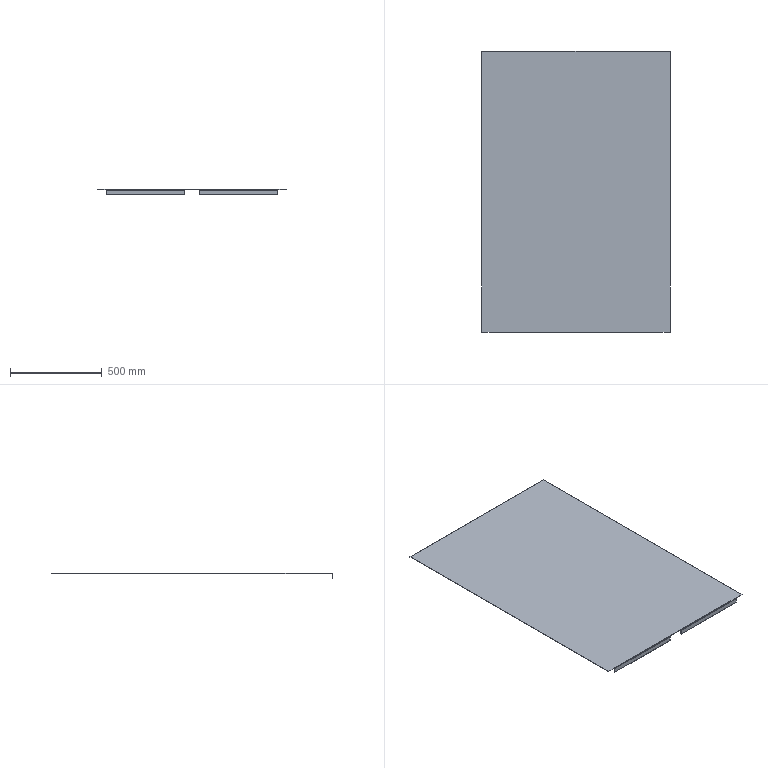Part | SolidWorks | features BaseBody 1 | 1 solid | 26 faces | box 1026 x 1530 x 27.5 mm | volume 3180339 mm3 | plane 22 | cylinder 4 | commonest cylinder face diameters 2 x2 6 x2
STEP:
#1=CARTESIAN_POINT('',(42.5,-764.5,-27.5));
#2=VERTEX_POINT('',#1);
#3=CARTESIAN_POINT('',(467.,-764.5,-27.5));
#4=VERTEX_POINT('',#3);
#5=CARTESIAN_POINT('',(467.,-764.5,-27.5));
#6=DIRECTION('',(1.,0.,0.));
#7=VECTOR('',#6,1000.);
#8=LINE('',#5,#7);
#9=EDGE_CURVE('',#2,#4,#8,.T.);
#10=ORIENTED_EDGE('',*,*,#9,.T.);
#11=CARTESIAN_POINT('',(467.,-766.5,-27.5));
#12=VERTEX_POINT('',#11);
#13=CARTESIAN_POINT('',(467.,-766.5,-27.5));
#14=DIRECTION('',(0.,1.,0.));
#15=VECTOR('',#14,1000.);
#16=LINE('',#13,#15);
#17=EDGE_CURVE('',#12,#4,#16,.T.);
#18=ORIENTED_EDGE('',*,*,#17,.F.);
#19=CARTESIAN_POINT('',(42.5,-766.5,-27.5));
#20=VERTEX_POINT('',#19);
#21=CARTESIAN_POINT('',(0.,-766.5,-27.5));
#22=DIRECTION('',(1.,0.,0.));
#23=VECTOR('',#22,1000.);
#24=LINE('',#21,#23);
#25=EDGE_CURVE('',#20,#12,#24,.T.);
#26=ORIENTED_EDGE('',*,*,#25,.F.);
#27=CARTESIAN_POINT('',(42.5,-766.5,-27.5));
#28=DIRECTION('',(0.,1.,0.));
#29=VECTOR('',#28,1000.);
#30=LINE('',#27,#29);
#31=EDGE_CURVE('',#20,#2,#30,.T.);
#32=ORIENTED_EDGE('',*,*,#31,.T.);
#33=EDGE_LOOP('',(#10,#18,#26,#32));
#34=FACE_OUTER_BOUND('',#33,.T.);
#35=CARTESIAN_POINT('',(467.,-766.5,-27.5));
#36=DIRECTION('',(0.,0.,1.));
#37=DIRECTION('',(0.,-1.,0.));
#38=AXIS2_PLACEMENT_3D('',#35,#36,#37);
#39=PLANE('',#38);
#40=ADVANCED_FACE('',(#34),#39,.F.);
#41=CARTESIAN_POINT('',(42.5,-764.5,-3.));
#42=VERTEX_POINT('',#41);
#43=CARTESIAN_POINT('',(42.5,-764.5,-2.));
#44=DIRECTION('',(0.,0.,-1.));
#45=VECTOR('',#44,1000.);
#46=LINE('',#43,#45);
#47=EDGE_CURVE('',#42,#2,#46,.T.);
#48=ORIENTED_EDGE('',*,*,#47,.F.);
#49=CARTESIAN_POINT('',(467.,-764.5,-3.));
#50=VERTEX_POINT('',#49);
#51=CARTESIAN_POINT('',(467.,-764.5,-3.));
#52=DIRECTION('',(-1.,0.,0.));
#53=VECTOR('',#52,1000.);
#54=LINE('',#51,#53);
#55=EDGE_CURVE('',#50,#42,#54,.T.);
#56=ORIENTED_EDGE('',*,*,#55,.F.);
#57=CARTESIAN_POINT('',(467.,-764.5,-2.));
#58=DIRECTION('',(0.,0.,1.));
#59=VECTOR('',#58,1000.);
#60=LINE('',#57,#59);
#61=EDGE_CURVE('',#4,#50,#60,.T.);
#62=ORIENTED_EDGE('',*,*,#61,.F.);
#63=ORIENTED_EDGE('',*,*,#9,.F.);
#64=EDGE_LOOP('',(#48,#56,#62,#63));
#65=FACE_OUTER_BOUND('',#64,.T.);
#66=CARTESIAN_POINT('',(0.,-764.5,0.));
#67=DIRECTION('',(0.,1.,0.));
#68=DIRECTION('',(0.,0.,-1.));
#69=AXIS2_PLACEMENT_3D('',#66,#67,#68);
#70=PLANE('',#69);
#71=ADVANCED_FACE('',(#65),#70,.T.);
#72=CARTESIAN_POINT('',(42.5,-766.5,-3.));
#73=VERTEX_POINT('',#72);
#74=CARTESIAN_POINT('',(467.,-766.5,-3.));
#75=VERTEX_POINT('',#74);
#76=CARTESIAN_POINT('',(467.,-766.5,-3.));
#77=DIRECTION('',(1.,0.,0.));
#78=VECTOR('',#77,1000.);
#79=LINE('',#76,#78);
#80=EDGE_CURVE('',#73,#75,#79,.T.);
#81=ORIENTED_EDGE('',*,*,#80,.F.);
#82=CARTESIAN_POINT('',(42.5,-766.5,0.));
#83=DIRECTION('',(0.,0.,-1.));
#84=VECTOR('',#83,1000.);
#85=LINE('',#82,#84);
#86=EDGE_CURVE('',#73,#20,#85,.T.);
#87=ORIENTED_EDGE('',*,*,#86,.T.);
#88=ORIENTED_EDGE('',*,*,#25,.T.);
#89=CARTESIAN_POINT('',(467.,-766.5,0.));
#90=DIRECTION('',(0.,0.,1.));
#91=VECTOR('',#90,1000.);
#92=LINE('',#89,#91);
#93=EDGE_CURVE('',#12,#75,#92,.T.);
#94=ORIENTED_EDGE('',*,*,#93,.T.);
#95=EDGE_LOOP('',(#81,#87,#88,#94));
#96=FACE_OUTER_BOUND('',#95,.T.);
#97=CARTESIAN_POINT('',(0.,-766.5,0.));
#98=DIRECTION('',(0.,1.,0.));
#99=DIRECTION('',(0.,0.,-1.));
#100=AXIS2_PLACEMENT_3D('',#97,#98,#99);
#101=PLANE('',#100);
#102=ADVANCED_FACE('',(#96),#101,.F.);
#103=CARTESIAN_POINT('',(467.,-766.5,-3.));
#104=DIRECTION('',(0.,-1.,0.));
#105=VECTOR('',#104,1000.);
#106=LINE('',#103,#105);
#107=EDGE_CURVE('',#50,#75,#106,.T.);
#108=ORIENTED_EDGE('',*,*,#107,.T.);
#109=ORIENTED_EDGE('',*,*,#93,.F.);
#110=ORIENTED_EDGE('',*,*,#17,.T.);
#111=ORIENTED_EDGE('',*,*,#61,.T.);
#112=EDGE_LOOP('',(#108,#109,#110,#111));
#113=FACE_OUTER_BOUND('',#112,.T.);
#114=CARTESIAN_POINT('',(467.,-766.5,-2.));
#115=DIRECTION('',(-1.,0.,0.));
#116=DIRECTION('',(0.,1.,0.));
#117=AXIS2_PLACEMENT_3D('',#114,#115,#116);
#118=PLANE('',#117);
#119=ADVANCED_FACE('',(#113),#118,.F.);
#120=CARTESIAN_POINT('',(42.5,-764.5,-3.));
#121=DIRECTION('',(0.,-1.,0.));
#122=VECTOR('',#121,1000.);
#123=LINE('',#120,#122);
#124=EDGE_CURVE('',#42,#73,#123,.T.);
#125=ORIENTED_EDGE('',*,*,#124,.F.);
#126=ORIENTED_EDGE('',*,*,#47,.T.);
#127=ORIENTED_EDGE('',*,*,#31,.F.);
#128=ORIENTED_EDGE('',*,*,#86,.F.);
#129=EDGE_LOOP('',(#125,#126,#127,#128));
#130=FACE_OUTER_BOUND('',#129,.T.);
#131=CARTESIAN_POINT('',(42.5,-766.5,-2.));
#132=DIRECTION('',(1.,0.,0.));
#133=DIRECTION('',(0.,1.,0.));
#134=AXIS2_PLACEMENT_3D('',#131,#132,#133);
#135=PLANE('',#134);
#136=ADVANCED_FACE('',(#130),#135,.F.);
#137=CARTESIAN_POINT('',(42.5,-763.5,-2.));
#138=VERTEX_POINT('',#137);
#139=CARTESIAN_POINT('',(467.,-763.5,-2.));
#140=VERTEX_POINT('',#139);
#141=CARTESIAN_POINT('',(42.5,-763.5,-2.));
#142=DIRECTION('',(1.,0.,0.));
#143=VECTOR('',#142,1000.);
#144=LINE('',#141,#143);
#145=EDGE_CURVE('',#138,#140,#144,.T.);
#146=ORIENTED_EDGE('',*,*,#145,.T.);
#147=CARTESIAN_POINT('',(467.,-763.5,-3.));
#148=DIRECTION('',(1.,0.,0.));
#149=DIRECTION('',(0.,0.,1.));
#150=AXIS2_PLACEMENT_3D('',#147,#148,#149);
#151=CIRCLE('',#150,1.);
#152=EDGE_CURVE('',#140,#50,#151,.T.);
#153=ORIENTED_EDGE('',*,*,#152,.T.);
#154=ORIENTED_EDGE('',*,*,#55,.T.);
#155=CARTESIAN_POINT('',(42.5,-763.5,-3.));
#156=DIRECTION('',(-1.,0.,0.));
#157=DIRECTION('',(0.,0.,1.));
#158=AXIS2_PLACEMENT_3D('',#155,#156,#157);
#159=CIRCLE('',#158,1.);
#160=EDGE_CURVE('',#42,#138,#159,.T.);
#161=ORIENTED_EDGE('',*,*,#160,.T.);
#162=EDGE_LOOP('',(#146,#153,#154,#161));
#163=FACE_OUTER_BOUND('',#162,.T.);
#164=CARTESIAN_POINT('',(42.5,-763.5,-3.));
#165=DIRECTION('',(-1.,0.,0.));
#166=DIRECTION('',(0.,-1.,0.));
#167=AXIS2_PLACEMENT_3D('',#164,#165,#166);
#168=CYLINDRICAL_SURFACE('',#167,1.);
#169=ADVANCED_FACE('',(#163),#168,.F.);
#170=CARTESIAN_POINT('',(42.5,-763.5,0.));
#171=VERTEX_POINT('',#170);
#172=CARTESIAN_POINT('',(467.,-763.5,0.));
#173=VERTEX_POINT('',#172);
#174=CARTESIAN_POINT('',(42.5,-763.5,0.));
#175=DIRECTION('',(1.,0.,0.));
#176=VECTOR('',#175,1000.);
#177=LINE('',#174,#176);
#178=EDGE_CURVE('',#171,#173,#177,.T.);
#179=ORIENTED_EDGE('',*,*,#178,.F.);
#180=CARTESIAN_POINT('',(42.5,-763.5,-3.));
#181=DIRECTION('',(-1.,0.,0.));
#182=DIRECTION('',(0.,0.,1.));
#183=AXIS2_PLACEMENT_3D('',#180,#181,#182);
#184=CIRCLE('',#183,3.);
#185=EDGE_CURVE('',#73,#171,#184,.T.);
#186=ORIENTED_EDGE('',*,*,#185,.F.);
#187=ORIENTED_EDGE('',*,*,#80,.T.);
#188=CARTESIAN_POINT('',(467.,-763.5,-3.));
#189=DIRECTION('',(1.,0.,0.));
#190=DIRECTION('',(0.,0.,1.));
#191=AXIS2_PLACEMENT_3D('',#188,#189,#190);
#192=CIRCLE('',#191,3.);
#193=EDGE_CURVE('',#173,#75,#192,.T.);
#194=ORIENTED_EDGE('',*,*,#193,.F.);
#195=EDGE_LOOP('',(#179,#186,#187,#194));
#196=FACE_OUTER_BOUND('',#195,.T.);
#197=CARTESIAN_POINT('',(42.5,-763.5,-3.));
#198=DIRECTION('',(-1.,0.,0.));
#199=DIRECTION('',(0.,-1.,0.));
#200=AXIS2_PLACEMENT_3D('',#197,#198,#199);
#201=CYLINDRICAL_SURFACE('',#200,3.);
#202=ADVANCED_FACE('',(#196),#201,.T.);
#203=ORIENTED_EDGE('',*,*,#160,.F.);
#204=ORIENTED_EDGE('',*,*,#124,.T.);
#205=ORIENTED_EDGE('',*,*,#185,.T.);
#206=CARTESIAN_POINT('',(42.5,-763.5,-2.));
#207=DIRECTION('',(0.,0.,1.));
#208=VECTOR('',#207,1000.);
#209=LINE('',#206,#208);
#210=EDGE_CURVE('',#138,#171,#209,.T.);
#211=ORIENTED_EDGE('',*,*,#210,.F.);
#212=EDGE_LOOP('',(#203,#204,#205,#211));
#213=FACE_OUTER_BOUND('',#212,.T.);
#214=CARTESIAN_POINT('',(42.5,-763.5,-3.));
#215=DIRECTION('',(1.,0.,0.));
#216=DIRECTION('',(0.,1.,0.));
#217=AXIS2_PLACEMENT_3D('',#214,#215,#216);
#218=PLANE('',#217);
#219=ADVANCED_FACE('',(#213),#218,.F.);
#220=ORIENTED_EDGE('',*,*,#107,.F.);
#221=ORIENTED_EDGE('',*,*,#152,.F.);
#222=CARTESIAN_POINT('',(467.,-763.5,-2.));
#223=DIRECTION('',(0.,0.,1.));
#224=VECTOR('',#223,1000.);
#225=LINE('',#222,#224);
#226=EDGE_CURVE('',#140,#173,#225,.T.);
#227=ORIENTED_EDGE('',*,*,#226,.T.);
#228=ORIENTED_EDGE('',*,*,#193,.T.);
#229=EDGE_LOOP('',(#220,#221,#227,#228));
#230=FACE_OUTER_BOUND('',#229,.T.);
#231=CARTESIAN_POINT('',(467.,-763.5,-3.));
#232=DIRECTION('',(1.,0.,0.));
#233=DIRECTION('',(0.,1.,0.));
#234=AXIS2_PLACEMENT_3D('',#231,#232,#233);
#235=PLANE('',#234);
#236=ADVANCED_FACE('',(#230),#235,.T.);
#237=CARTESIAN_POINT('',(-42.5,-764.5,-27.5));
#238=VERTEX_POINT('',#237);
#239=CARTESIAN_POINT('',(-467.,-764.5,-27.5));
#240=VERTEX_POINT('',#239);
#241=CARTESIAN_POINT('',(0.,-764.5,-27.5));
#242=DIRECTION('',(-1.,0.,0.));
#243=VECTOR('',#242,1000.);
#244=LINE('',#241,#243);
#245=EDGE_CURVE('',#238,#240,#244,.T.);
#246=ORIENTED_EDGE('',*,*,#245,.F.);
#247=CARTESIAN_POINT('',(-42.5,-766.5,-27.5));
#248=VERTEX_POINT('',#247);
#249=CARTESIAN_POINT('',(-42.5,-766.5,-27.5));
#250=DIRECTION('',(0.,1.,0.));
#251=VECTOR('',#250,1000.);
#252=LINE('',#249,#251);
#253=EDGE_CURVE('',#248,#238,#252,.T.);
#254=ORIENTED_EDGE('',*,*,#253,.F.);
#255=CARTESIAN_POINT('',(-467.,-766.5,-27.5));
#256=VERTEX_POINT('',#255);
#257=CARTESIAN_POINT('',(-467.,-766.5,-27.5));
#258=DIRECTION('',(-1.,0.,0.));
#259=VECTOR('',#258,1000.);
#260=LINE('',#257,#259);
#261=EDGE_CURVE('',#248,#256,#260,.T.);
#262=ORIENTED_EDGE('',*,*,#261,.T.);
#263=CARTESIAN_POINT('',(-467.,-766.5,-27.5));
#264=DIRECTION('',(0.,1.,0.));
#265=VECTOR('',#264,1000.);
#266=LINE('',#263,#265);
#267=EDGE_CURVE('',#256,#240,#266,.T.);
#268=ORIENTED_EDGE('',*,*,#267,.T.);
#269=EDGE_LOOP('',(#246,#254,#262,#268));
#270=FACE_OUTER_BOUND('',#269,.T.);
#271=CARTESIAN_POINT('',(-467.,-766.5,-27.5));
#272=DIRECTION('',(0.,0.,-1.));
#273=DIRECTION('',(0.,-1.,0.));
#274=AXIS2_PLACEMENT_3D('',#271,#272,#273);
#275=PLANE('',#274);
#276=ADVANCED_FACE('',(#270),#275,.T.);
#277=CARTESIAN_POINT('',(-42.5,-764.5,-3.));
#278=VERTEX_POINT('',#277);
#279=CARTESIAN_POINT('',(-467.,-764.5,-3.));
#280=VERTEX_POINT('',#279);
#281=CARTESIAN_POINT('',(-42.5,-764.5,-3.));
#282=DIRECTION('',(-1.,0.,0.));
#283=VECTOR('',#282,1000.);
#284=LINE('',#281,#283);
#285=EDGE_CURVE('',#278,#280,#284,.T.);
#286=ORIENTED_EDGE('',*,*,#285,.F.);
#287=CARTESIAN_POINT('',(-42.5,-764.5,0.));
#288=DIRECTION('',(0.,0.,-1.));
#289=VECTOR('',#288,1000.);
#290=LINE('',#287,#289);
#291=EDGE_CURVE('',#278,#238,#290,.T.);
#292=ORIENTED_EDGE('',*,*,#291,.T.);
#293=ORIENTED_EDGE('',*,*,#245,.T.);
#294=CARTESIAN_POINT('',(-467.,-764.5,0.));
#295=DIRECTION('',(0.,0.,1.));
#296=VECTOR('',#295,1000.);
#297=LINE('',#294,#296);
#298=EDGE_CURVE('',#240,#280,#297,.T.);
#299=ORIENTED_EDGE('',*,*,#298,.T.);
#300=EDGE_LOOP('',(#286,#292,#293,#299));
#301=FACE_OUTER_BOUND('',#300,.T.);
#302=CARTESIAN_POINT('',(0.,-764.5,0.));
#303=DIRECTION('',(0.,-1.,0.));
#304=DIRECTION('',(-1.,0.,0.));
#305=AXIS2_PLACEMENT_3D('',#302,#303,#304);
#306=PLANE('',#305);
#307=ADVANCED_FACE('',(#301),#306,.F.);
#308=CARTESIAN_POINT('',(-42.5,-766.5,-3.));
#309=VERTEX_POINT('',#308);
#310=CARTESIAN_POINT('',(-42.5,-766.5,-2.));
#311=DIRECTION('',(0.,0.,-1.));
#312=VECTOR('',#311,1000.);
#313=LINE('',#310,#312);
#314=EDGE_CURVE('',#309,#248,#313,.T.);
#315=ORIENTED_EDGE('',*,*,#314,.F.);
#316=CARTESIAN_POINT('',(-467.,-766.5,-3.));
#317=VERTEX_POINT('',#316);
#318=CARTESIAN_POINT('',(0.,-766.5,-3.));
#319=DIRECTION('',(-1.,0.,0.));
#320=VECTOR('',#319,1000.);
#321=LINE('',#318,#320);
#322=EDGE_CURVE('',#309,#317,#321,.T.);
#323=ORIENTED_EDGE('',*,*,#322,.T.);
#324=CARTESIAN_POINT('',(-467.,-766.5,-2.));
#325=DIRECTION('',(0.,0.,1.));
#326=VECTOR('',#325,1000.);
#327=LINE('',#324,#326);
#328=EDGE_CURVE('',#256,#317,#327,.T.);
#329=ORIENTED_EDGE('',*,*,#328,.F.);
#330=ORIENTED_EDGE('',*,*,#261,.F.);
#331=EDGE_LOOP('',(#315,#323,#329,#330));
#332=FACE_OUTER_BOUND('',#331,.T.);
#333=CARTESIAN_POINT('',(0.,-766.5,0.));
#334=DIRECTION('',(0.,-1.,0.));
#335=DIRECTION('',(-1.,0.,0.));
#336=AXIS2_PLACEMENT_3D('',#333,#334,#335);
#337=PLANE('',#336);
#338=ADVANCED_FACE('',(#332),#337,.T.);
#339=ORIENTED_EDGE('',*,*,#328,.T.);
#340=CARTESIAN_POINT('',(-467.,-764.5,-3.));
#341=DIRECTION('',(0.,-1.,0.));
#342=VECTOR('',#341,1000.);
#343=LINE('',#340,#342);
#344=EDGE_CURVE('',#280,#317,#343,.T.);
#345=ORIENTED_EDGE('',*,*,#344,.F.);
#346=ORIENTED_EDGE('',*,*,#298,.F.);
#347=ORIENTED_EDGE('',*,*,#267,.F.);
#348=EDGE_LOOP('',(#339,#345,#346,#347));
#349=FACE_OUTER_BOUND('',#348,.T.);
#350=CARTESIAN_POINT('',(-467.,-766.5,-2.));
#351=DIRECTION('',(-1.,0.,0.));
#352=DIRECTION('',(0.,1.,0.));
#353=AXIS2_PLACEMENT_3D('',#350,#351,#352);
#354=PLANE('',#353);
#355=ADVANCED_FACE('',(#349),#354,.T.);
#356=ORIENTED_EDGE('',*,*,#291,.F.);
#357=CARTESIAN_POINT('',(-42.5,-766.5,-3.));
#358=DIRECTION('',(0.,-1.,0.));
#359=VECTOR('',#358,1000.);
#360=LINE('',#357,#359);
#361=EDGE_CURVE('',#278,#309,#360,.T.);
#362=ORIENTED_EDGE('',*,*,#361,.T.);
#363=ORIENTED_EDGE('',*,*,#314,.T.);
#364=ORIENTED_EDGE('',*,*,#253,.T.);
#365=EDGE_LOOP('',(#356,#362,#363,#364));
#366=FACE_OUTER_BOUND('',#365,.T.);
#367=CARTESIAN_POINT('',(-42.5,-766.5,-2.));
#368=DIRECTION('',(1.,0.,0.));
#369=DIRECTION('',(0.,1.,0.));
#370=AXIS2_PLACEMENT_3D('',#367,#368,#369);
#371=PLANE('',#370);
#372=ADVANCED_FACE('',(#366),#371,.T.);
#373=CARTESIAN_POINT('',(-467.,-763.5,-2.));
#374=VERTEX_POINT('',#373);
#375=CARTESIAN_POINT('',(-42.5,-763.5,-2.));
#376=VERTEX_POINT('',#375);
#377=CARTESIAN_POINT('',(-467.,-763.5,-2.));
#378=DIRECTION('',(1.,0.,0.));
#379=VECTOR('',#378,1000.);
#380=LINE('',#377,#379);
#381=EDGE_CURVE('',#374,#376,#380,.T.);
#382=ORIENTED_EDGE('',*,*,#381,.T.);
#383=CARTESIAN_POINT('',(-42.5,-763.5,-3.));
#384=DIRECTION('',(1.,0.,0.));
#385=DIRECTION('',(0.,0.,1.));
#386=AXIS2_PLACEMENT_3D('',#383,#384,#385);
#387=CIRCLE('',#386,1.);
#388=EDGE_CURVE('',#376,#278,#387,.T.);
#389=ORIENTED_EDGE('',*,*,#388,.T.);
#390=ORIENTED_EDGE('',*,*,#285,.T.);
#391=CARTESIAN_POINT('',(-467.,-763.5,-3.));
#392=DIRECTION('',(-1.,0.,0.));
#393=DIRECTION('',(0.,0.,1.));
#394=AXIS2_PLACEMENT_3D('',#391,#392,#393);
#395=CIRCLE('',#394,1.);
#396=EDGE_CURVE('',#280,#374,#395,.T.);
#397=ORIENTED_EDGE('',*,*,#396,.T.);
#398=EDGE_LOOP('',(#382,#389,#390,#397));
#399=FACE_OUTER_BOUND('',#398,.T.);
#400=CARTESIAN_POINT('',(-467.,-763.5,-3.));
#401=DIRECTION('',(-1.,0.,0.));
#402=DIRECTION('',(0.,-1.,0.));
#403=AXIS2_PLACEMENT_3D('',#400,#401,#402);
#404=CYLINDRICAL_SURFACE('',#403,1.);
#405=ADVANCED_FACE('',(#399),#404,.F.);
#406=CARTESIAN_POINT('',(-467.,-763.5,0.));
#407=VERTEX_POINT('',#406);
#408=CARTESIAN_POINT('',(-42.5,-763.5,0.));
#409=VERTEX_POINT('',#408);
#410=CARTESIAN_POINT('',(-467.,-763.5,0.));
#411=DIRECTION('',(1.,0.,0.));
#412=VECTOR('',#411,1000.);
#413=LINE('',#410,#412);
#414=EDGE_CURVE('',#407,#409,#413,.T.);
#415=ORIENTED_EDGE('',*,*,#414,.F.);
#416=CARTESIAN_POINT('',(-467.,-763.5,-3.));
#417=DIRECTION('',(-1.,0.,0.));
#418=DIRECTION('',(0.,0.,1.));
#419=AXIS2_PLACEMENT_3D('',#416,#417,#418);
#420=CIRCLE('',#419,3.);
#421=EDGE_CURVE('',#317,#407,#420,.T.);
#422=ORIENTED_EDGE('',*,*,#421,.F.);
#423=ORIENTED_EDGE('',*,*,#322,.F.);
#424=CARTESIAN_POINT('',(-42.5,-763.5,-3.));
#425=DIRECTION('',(1.,0.,0.));
#426=DIRECTION('',(0.,0.,1.));
#427=AXIS2_PLACEMENT_3D('',#424,#425,#426);
#428=CIRCLE('',#427,3.);
#429=EDGE_CURVE('',#409,#309,#428,.T.);
#430=ORIENTED_EDGE('',*,*,#429,.F.);
#431=EDGE_LOOP('',(#415,#422,#423,#430));
#432=FACE_OUTER_BOUND('',#431,.T.);
#433=CARTESIAN_POINT('',(-467.,-763.5,-3.));
#434=DIRECTION('',(-1.,0.,0.));
#435=DIRECTION('',(0.,-1.,0.));
#436=AXIS2_PLACEMENT_3D('',#433,#434,#435);
#437=CYLINDRICAL_SURFACE('',#436,3.);
#438=ADVANCED_FACE('',(#432),#437,.T.);
#439=ORIENTED_EDGE('',*,*,#396,.F.);
#440=ORIENTED_EDGE('',*,*,#344,.T.);
#441=ORIENTED_EDGE('',*,*,#421,.T.);
#442=CARTESIAN_POINT('',(-467.,-763.5,-2.));
#443=DIRECTION('',(0.,0.,1.));
#444=VECTOR('',#443,1000.);
#445=LINE('',#442,#444);
#446=EDGE_CURVE('',#374,#407,#445,.T.);
#447=ORIENTED_EDGE('',*,*,#446,.F.);
#448=EDGE_LOOP('',(#439,#440,#441,#447));
#449=FACE_OUTER_BOUND('',#448,.T.);
#450=CARTESIAN_POINT('',(-467.,-763.5,-3.));
#451=DIRECTION('',(1.,0.,0.));
#452=DIRECTION('',(0.,1.,0.));
#453=AXIS2_PLACEMENT_3D('',#450,#451,#452);
#454=PLANE('',#453);
#455=ADVANCED_FACE('',(#449),#454,.F.);
#456=ORIENTED_EDGE('',*,*,#361,.F.);
#457=ORIENTED_EDGE('',*,*,#388,.F.);
#458=CARTESIAN_POINT('',(-42.5,-763.5,-2.));
#459=DIRECTION('',(0.,0.,1.));
#460=VECTOR('',#459,1000.);
#461=LINE('',#458,#460);
#462=EDGE_CURVE('',#376,#409,#461,.T.);
#463=ORIENTED_EDGE('',*,*,#462,.T.);
#464=ORIENTED_EDGE('',*,*,#429,.T.);
#465=EDGE_LOOP('',(#456,#457,#463,#464));
#466=FACE_OUTER_BOUND('',#465,.T.);
#467=CARTESIAN_POINT('',(-42.5,-763.5,-3.));
#468=DIRECTION('',(1.,0.,0.));
#469=DIRECTION('',(0.,1.,0.));
#470=AXIS2_PLACEMENT_3D('',#467,#468,#469);
#471=PLANE('',#470);
#472=ADVANCED_FACE('',(#466),#471,.T.);
#473=CARTESIAN_POINT('',(-513.,763.5,0.));
#474=VERTEX_POINT('',#473);
#475=CARTESIAN_POINT('',(-513.,-763.5,0.));
#476=VERTEX_POINT('',#475);
#477=CARTESIAN_POINT('',(-513.,763.5,0.));
#478=DIRECTION('',(0.,-1.,0.));
#479=VECTOR('',#478,1000.);
#480=LINE('',#477,#479);
#481=EDGE_CURVE('',#474,#476,#480,.T.);
#482=ORIENTED_EDGE('',*,*,#481,.T.);
#483=CARTESIAN_POINT('',(513.,-763.5,0.));
#484=DIRECTION('',(1.,0.,0.));
#485=VECTOR('',#484,1000.);
#486=LINE('',#483,#485);
#487=EDGE_CURVE('',#476,#407,#486,.T.);
#488=ORIENTED_EDGE('',*,*,#487,.T.);
#489=ORIENTED_EDGE('',*,*,#414,.T.);
#490=CARTESIAN_POINT('',(513.,-763.5,0.));
#491=DIRECTION('',(1.,0.,0.));
#492=VECTOR('',#491,1000.);
#493=LINE('',#490,#492);
#494=EDGE_CURVE('',#409,#171,#493,.T.);
#495=ORIENTED_EDGE('',*,*,#494,.T.);
#496=ORIENTED_EDGE('',*,*,#178,.T.);
#497=CARTESIAN_POINT('',(513.,-763.5,0.));
#498=VERTEX_POINT('',#497);
#499=CARTESIAN_POINT('',(513.,-763.5,0.));
#500=DIRECTION('',(1.,0.,0.));
#501=VECTOR('',#500,1000.);
#502=LINE('',#499,#501);
#503=EDGE_CURVE('',#173,#498,#502,.T.);
#504=ORIENTED_EDGE('',*,*,#503,.T.);
#505=CARTESIAN_POINT('',(513.,763.5,0.));
#506=VERTEX_POINT('',#505);
#507=CARTESIAN_POINT('',(513.,763.5,0.));
#508=DIRECTION('',(0.,1.,0.));
#509=VECTOR('',#508,1000.);
#510=LINE('',#507,#509);
#511=EDGE_CURVE('',#498,#506,#510,.T.);
#512=ORIENTED_EDGE('',*,*,#511,.T.);
#513=CARTESIAN_POINT('',(513.,763.5,0.));
#514=DIRECTION('',(-1.,0.,0.));
#515=VECTOR('',#514,1000.);
#516=LINE('',#513,#515);
#517=EDGE_CURVE('',#506,#474,#516,.T.);
#518=ORIENTED_EDGE('',*,*,#517,.T.);
#519=EDGE_LOOP('',(#482,#488,#489,#495,#496,#504,#512,#518));
#520=FACE_OUTER_BOUND('',#519,.T.);
#521=CARTESIAN_POINT('',(0.,0.,0.));
#522=DIRECTION('',(0.,0.,-1.));
#523=DIRECTION('',(0.,-1.,0.));
#524=AXIS2_PLACEMENT_3D('',#521,#522,#523);
#525=PLANE('',#524);
#526=ADVANCED_FACE('',(#520),#525,.F.);
#527=CARTESIAN_POINT('',(-513.,763.5,-2.));
#528=VERTEX_POINT('',#527);
#529=CARTESIAN_POINT('',(-513.,-763.5,-2.));
#530=VERTEX_POINT('',#529);
#531=CARTESIAN_POINT('',(-513.,763.5,-2.));
#532=DIRECTION('',(0.,-1.,0.));
#533=VECTOR('',#532,1000.);
#534=LINE('',#531,#533);
#535=EDGE_CURVE('',#528,#530,#534,.T.);
#536=ORIENTED_EDGE('',*,*,#535,.F.);
#537=CARTESIAN_POINT('',(513.,763.5,-2.));
#538=VERTEX_POINT('',#537);
#539=CARTESIAN_POINT('',(513.,763.5,-2.));
#540=DIRECTION('',(-1.,0.,0.));
#541=VECTOR('',#540,1000.);
#542=LINE('',#539,#541);
#543=EDGE_CURVE('',#538,#528,#542,.T.);
#544=ORIENTED_EDGE('',*,*,#543,.F.);
#545=CARTESIAN_POINT('',(513.,-763.5,-2.));
#546=VERTEX_POINT('',#545);
#547=CARTESIAN_POINT('',(513.,763.5,-2.));
#548=DIRECTION('',(0.,1.,0.));
#549=VECTOR('',#548,1000.);
#550=LINE('',#547,#549);
#551=EDGE_CURVE('',#546,#538,#550,.T.);
#552=ORIENTED_EDGE('',*,*,#551,.F.);
#553=CARTESIAN_POINT('',(513.,-763.5,-2.));
#554=DIRECTION('',(1.,0.,0.));
#555=VECTOR('',#554,1000.);
#556=LINE('',#553,#555);
#557=EDGE_CURVE('',#140,#546,#556,.T.);
#558=ORIENTED_EDGE('',*,*,#557,.F.);
#559=ORIENTED_EDGE('',*,*,#145,.F.);
#560=CARTESIAN_POINT('',(513.,-763.5,-2.));
#561=DIRECTION('',(1.,0.,0.));
#562=VECTOR('',#561,1000.);
#563=LINE('',#560,#562);
#564=EDGE_CURVE('',#376,#138,#563,.T.);
#565=ORIENTED_EDGE('',*,*,#564,.F.);
#566=ORIENTED_EDGE('',*,*,#381,.F.);
#567=CARTESIAN_POINT('',(513.,-763.5,-2.));
#568=DIRECTION('',(1.,0.,0.));
#569=VECTOR('',#568,1000.);
#570=LINE('',#567,#569);
#571=EDGE_CURVE('',#530,#374,#570,.T.);
#572=ORIENTED_EDGE('',*,*,#571,.F.);
#573=EDGE_LOOP('',(#536,#544,#552,#558,#559,#565,#566,#572));
#574=FACE_OUTER_BOUND('',#573,.T.);
#575=CARTESIAN_POINT('',(0.,0.,-2.));
#576=DIRECTION('',(0.,0.,-1.));
#577=DIRECTION('',(0.,-1.,0.));
#578=AXIS2_PLACEMENT_3D('',#575,#576,#577);
#579=PLANE('',#578);
#580=ADVANCED_FACE('',(#574),#579,.T.);
#581=ORIENTED_EDGE('',*,*,#226,.F.);
#582=ORIENTED_EDGE('',*,*,#557,.T.);
#583=CARTESIAN_POINT('',(513.,-763.5,-2.));
#584=DIRECTION('',(0.,0.,1.));
#585=VECTOR('',#584,1000.);
#586=LINE('',#583,#585);
#587=EDGE_CURVE('',#546,#498,#586,.T.);
#588=ORIENTED_EDGE('',*,*,#587,.T.);
#589=ORIENTED_EDGE('',*,*,#503,.F.);
#590=EDGE_LOOP('',(#581,#582,#588,#589));
#591=FACE_OUTER_BOUND('',#590,.T.);
#592=CARTESIAN_POINT('',(513.,-763.5,-2.));
#593=DIRECTION('',(0.,-1.,0.));
#594=DIRECTION('',(0.,0.,-1.));
#595=AXIS2_PLACEMENT_3D('',#592,#593,#594);
#596=PLANE('',#595);
#597=ADVANCED_FACE('',(#591),#596,.T.);
#598=ORIENTED_EDGE('',*,*,#511,.F.);
#599=ORIENTED_EDGE('',*,*,#587,.F.);
#600=ORIENTED_EDGE('',*,*,#551,.T.);
#601=CARTESIAN_POINT('',(513.,763.5,-2.));
#602=DIRECTION('',(0.,0.,1.));
#603=VECTOR('',#602,1000.);
#604=LINE('',#601,#603);
#605=EDGE_CURVE('',#538,#506,#604,.T.);
#606=ORIENTED_EDGE('',*,*,#605,.T.);
#607=EDGE_LOOP('',(#598,#599,#600,#606));
#608=FACE_OUTER_BOUND('',#607,.T.);
#609=CARTESIAN_POINT('',(513.,763.5,-2.));
#610=DIRECTION('',(1.,0.,0.));
#611=DIRECTION('',(0.,1.,0.));
#612=AXIS2_PLACEMENT_3D('',#609,#610,#611);
#613=PLANE('',#612);
#614=ADVANCED_FACE('',(#608),#613,.T.);
#615=ORIENTED_EDGE('',*,*,#517,.F.);
#616=ORIENTED_EDGE('',*,*,#605,.F.);
#617=ORIENTED_EDGE('',*,*,#543,.T.);
#618=CARTESIAN_POINT('',(-513.,763.5,-2.));
#619=DIRECTION('',(0.,0.,1.));
#620=VECTOR('',#619,1000.);
#621=LINE('',#618,#620);
#622=EDGE_CURVE('',#528,#474,#621,.T.);
#623=ORIENTED_EDGE('',*,*,#622,.T.);
#624=EDGE_LOOP('',(#615,#616,#617,#623));
#625=FACE_OUTER_BOUND('',#624,.T.);
#626=CARTESIAN_POINT('',(513.,763.5,-2.));
#627=DIRECTION('',(0.,1.,0.));
#628=DIRECTION('',(1.,0.,0.));
#629=AXIS2_PLACEMENT_3D('',#626,#627,#628);
#630=PLANE('',#629);
#631=ADVANCED_FACE('',(#625),#630,.T.);
#632=ORIENTED_EDGE('',*,*,#481,.F.);
#633=ORIENTED_EDGE('',*,*,#622,.F.);
#634=ORIENTED_EDGE('',*,*,#535,.T.);
#635=CARTESIAN_POINT('',(-513.,-763.5,-2.));
#636=DIRECTION('',(0.,0.,1.));
#637=VECTOR('',#636,1000.);
#638=LINE('',#635,#637);
#639=EDGE_CURVE('',#530,#476,#638,.T.);
#640=ORIENTED_EDGE('',*,*,#639,.T.);
#641=EDGE_LOOP('',(#632,#633,#634,#640));
#642=FACE_OUTER_BOUND('',#641,.T.);
#643=CARTESIAN_POINT('',(-513.,763.5,-2.));
#644=DIRECTION('',(-1.,0.,0.));
#645=DIRECTION('',(0.,1.,0.));
#646=AXIS2_PLACEMENT_3D('',#643,#644,#645);
#647=PLANE('',#646);
#648=ADVANCED_FACE('',(#642),#647,.T.);
#649=ORIENTED_EDGE('',*,*,#571,.T.);
#650=ORIENTED_EDGE('',*,*,#446,.T.);
#651=ORIENTED_EDGE('',*,*,#487,.F.);
#652=ORIENTED_EDGE('',*,*,#639,.F.);
#653=EDGE_LOOP('',(#649,#650,#651,#652));
#654=FACE_OUTER_BOUND('',#653,.T.);
#655=CARTESIAN_POINT('',(513.,-763.5,-2.));
#656=DIRECTION('',(0.,-1.,0.));
#657=DIRECTION('',(0.,0.,-1.));
#658=AXIS2_PLACEMENT_3D('',#655,#656,#657);
#659=PLANE('',#658);
#660=ADVANCED_FACE('',(#654),#659,.T.);
#661=ORIENTED_EDGE('',*,*,#564,.T.);
#662=ORIENTED_EDGE('',*,*,#210,.T.);
#663=ORIENTED_EDGE('',*,*,#494,.F.);
#664=ORIENTED_EDGE('',*,*,#462,.F.);
#665=EDGE_LOOP('',(#661,#662,#663,#664));
#666=FACE_OUTER_BOUND('',#665,.T.);
#667=CARTESIAN_POINT('',(513.,-763.5,-2.));
#668=DIRECTION('',(0.,-1.,0.));
#669=DIRECTION('',(0.,0.,-1.));
#670=AXIS2_PLACEMENT_3D('',#667,#668,#669);
#671=PLANE('',#670);
#672=ADVANCED_FACE('',(#666),#671,.T.);
#673=CLOSED_SHELL('',(#40,#71,#102,#119,#136,#169,#202,#219,#236,#276,#307,#338,#355,#372,#405,#438,#455,#472,#526,#580,#597,#614,#631,#648,#660,#672));
#674=MANIFOLD_SOLID_BREP('',#673);
#675=CARTESIAN_POINT('',(0.,0.,0.));
#676=DIRECTION('',(0.,0.,1.));
#677=DIRECTION('',(1.,0.,0.));
#678=AXIS2_PLACEMENT_3D('',#675,#676,#677);
#679=(LENGTH_UNIT()NAMED_UNIT(*)SI_UNIT(.MILLI.,.METRE.));
#680=UNCERTAINTY_MEASURE_WITH_UNIT(LENGTH_MEASURE(0.00001),#679,'','');
#681=(NAMED_UNIT(*)PLANE_ANGLE_UNIT()SI_UNIT($,.RADIAN.));
#682=(NAMED_UNIT(*)SI_UNIT($,.STERADIAN.)SOLID_ANGLE_UNIT());
#683=(GEOMETRIC_REPRESENTATION_CONTEXT(3)GLOBAL_UNCERTAINTY_ASSIGNED_CONTEXT((#680))GLOBAL_UNIT_ASSIGNED_CONTEXT((#679,#681,#682))REPRESENTATION_CONTEXT('',''));
#684=ADVANCED_BREP_SHAPE_REPRESENTATION('',(#674,#678),#683);